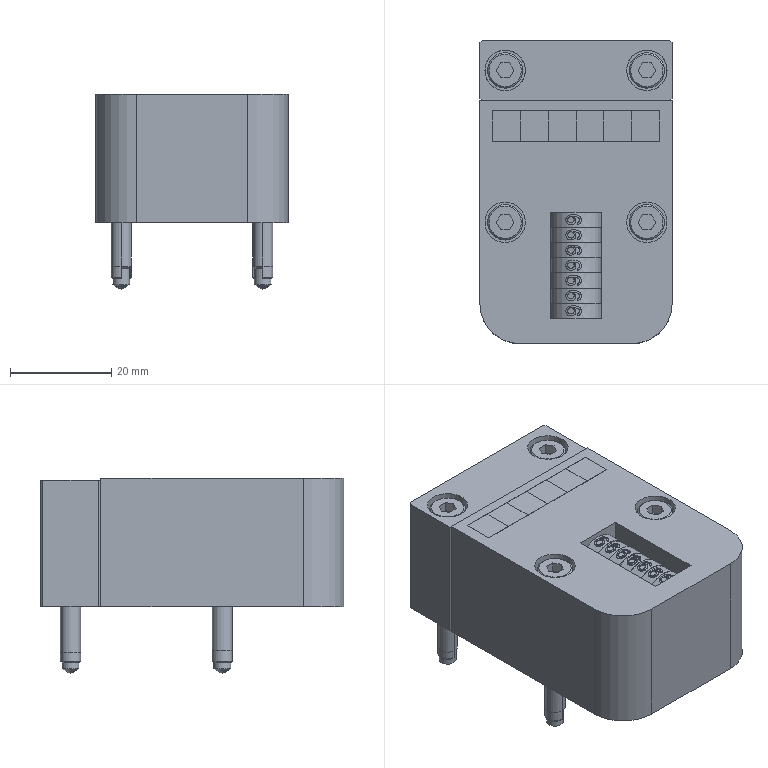Part | STEP file | E042000001 | 10 solids | 455 faces | box 38 x 60 x 38.607 mm | volume 56849 mm3 | plane 223 | other 148 | cylinder 52 | cone 32 | commonest cylinder face diameters 4 x8 10 x8 10.2 x7 9.8 x6 3.333 x4 3.987 x4